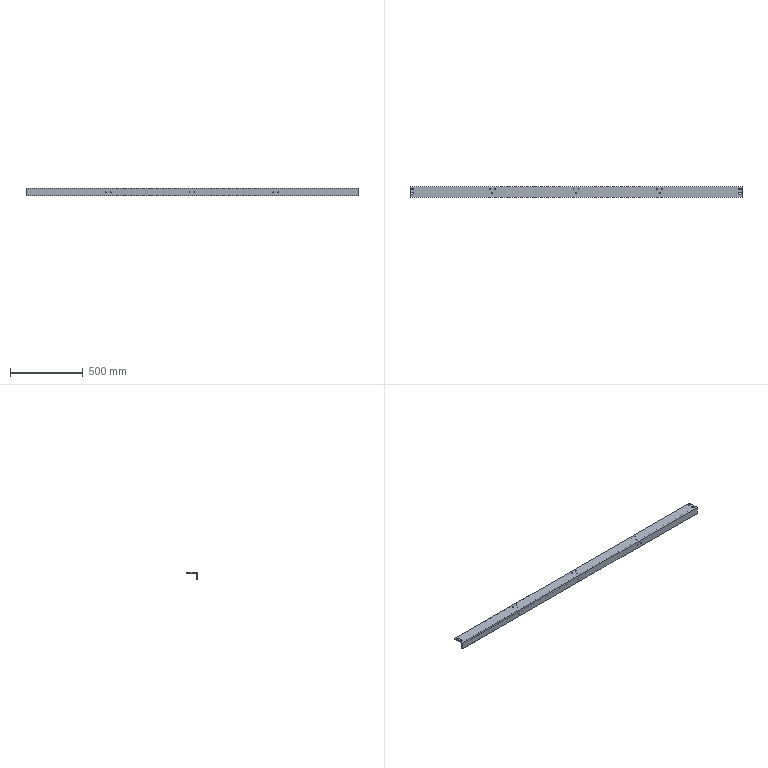Part | SolidWorks | features HoleWzd 2, Cut 1, WeldMemberFeat 1, WeldmentFeature 1 | 1 solid | 57 faces | box 2276 x 75 x 50 mm | volume 1389503 mm3 | cylinder 41 | plane 16 | commonest cylinder face diameters 5 x30 10 x8 3.333 x2 16 x1